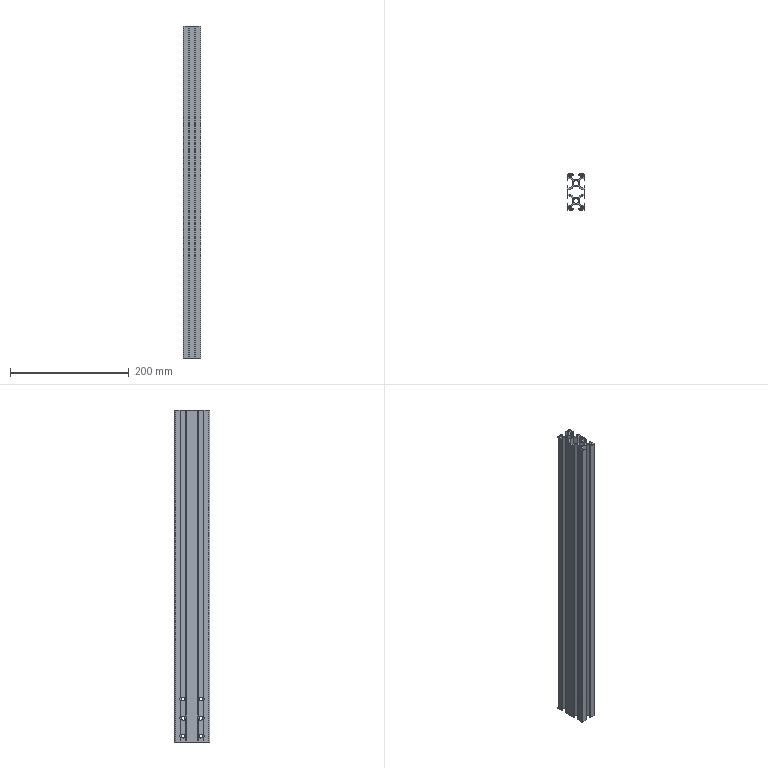Part | SolidWorks | features HoleWzd 1, WeldMemberFeat 1, WeldmentFeature 1 | 1 solid | 198 faces | box 30 x 60 x 560 mm | volume 279456 mm3 | plane 154 | cylinder 44 | commonest cylinder face diameters 6.6 x24 11 x12 9.2 x4 3 x2 5 x2